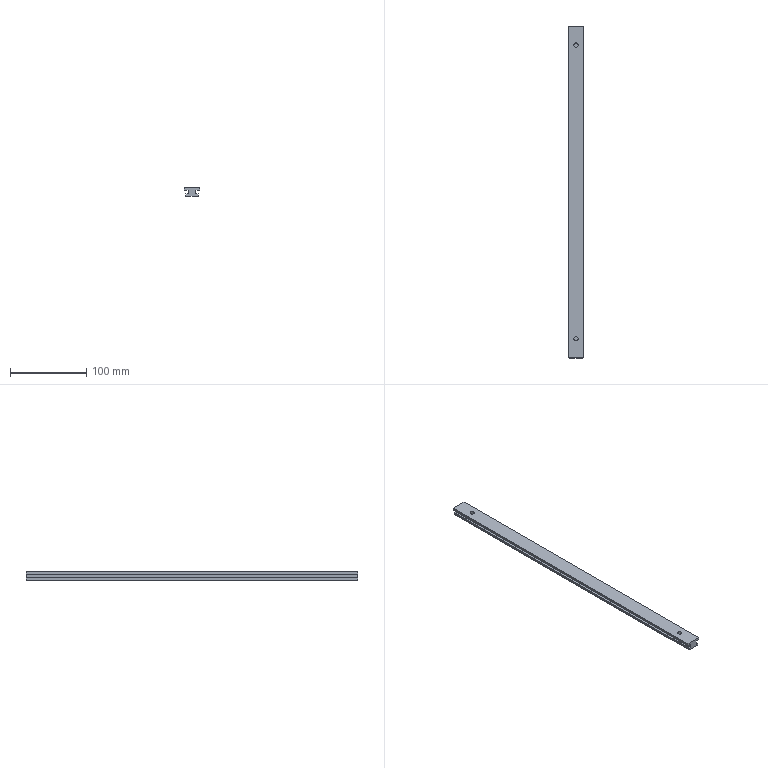Part | SolidWorks | features Extrusion 1, ICE 1 | 1 solid | 20 faces | box 20 x 435 x 11 mm | volume 68492 mm3 | plane 16 | cylinder 4 | commonest cylinder face diameters 5.5 x4
STEP:
#1=CARTESIAN_POINT('',(7.25,410.,-5.));
#2=VERTEX_POINT('',#1);
#3=CARTESIAN_POINT('',(12.75,410.,-5.));
#4=VERTEX_POINT('',#3);
#5=CARTESIAN_POINT('',(10.,410.,-5.));
#6=DIRECTION('',(0.,0.,1.));
#7=DIRECTION('',(1.,0.,0.));
#8=AXIS2_PLACEMENT_3D('',#5,#6,#7);
#9=CIRCLE('',#8,2.75);
#10=EDGE_CURVE('',#2,#4,#9,.T.);
#11=ORIENTED_EDGE('',*,*,#10,.F.);
#12=CARTESIAN_POINT('',(7.25,410.,0.));
#13=VERTEX_POINT('',#12);
#14=CARTESIAN_POINT('',(7.25,410.,-5.));
#15=DIRECTION('',(0.,0.,1.));
#16=VECTOR('',#15,1000.);
#17=LINE('',#14,#16);
#18=EDGE_CURVE('',#2,#13,#17,.T.);
#19=ORIENTED_EDGE('',*,*,#18,.T.);
#20=CARTESIAN_POINT('',(12.75,410.,0.));
#21=VERTEX_POINT('',#20);
#22=CARTESIAN_POINT('',(10.,410.,0.));
#23=DIRECTION('',(0.,0.,1.));
#24=DIRECTION('',(1.,0.,0.));
#25=AXIS2_PLACEMENT_3D('',#22,#23,#24);
#26=CIRCLE('',#25,2.75);
#27=EDGE_CURVE('',#13,#21,#26,.T.);
#28=ORIENTED_EDGE('',*,*,#27,.T.);
#29=CARTESIAN_POINT('',(12.75,410.,-5.));
#30=DIRECTION('',(0.,0.,1.));
#31=VECTOR('',#30,1000.);
#32=LINE('',#29,#31);
#33=EDGE_CURVE('',#4,#21,#32,.T.);
#34=ORIENTED_EDGE('',*,*,#33,.F.);
#35=EDGE_LOOP('',(#11,#19,#28,#34));
#36=FACE_OUTER_BOUND('',#35,.T.);
#37=CARTESIAN_POINT('',(10.,410.,-5.));
#38=DIRECTION('',(0.,0.,1.));
#39=DIRECTION('',(1.,0.,0.));
#40=AXIS2_PLACEMENT_3D('',#37,#38,#39);
#41=CYLINDRICAL_SURFACE('',#40,2.75);
#42=ADVANCED_FACE('',(#36),#41,.F.);
#43=CARTESIAN_POINT('',(7.25,25.,-5.));
#44=VERTEX_POINT('',#43);
#45=CARTESIAN_POINT('',(12.75,25.,-5.));
#46=VERTEX_POINT('',#45);
#47=CARTESIAN_POINT('',(10.,25.,-5.));
#48=DIRECTION('',(0.,0.,1.));
#49=DIRECTION('',(1.,0.,0.));
#50=AXIS2_PLACEMENT_3D('',#47,#48,#49);
#51=CIRCLE('',#50,2.75);
#52=EDGE_CURVE('',#44,#46,#51,.T.);
#53=ORIENTED_EDGE('',*,*,#52,.F.);
#54=CARTESIAN_POINT('',(7.25,25.,0.));
#55=VERTEX_POINT('',#54);
#56=CARTESIAN_POINT('',(7.25,25.,-5.));
#57=DIRECTION('',(0.,0.,1.));
#58=VECTOR('',#57,1000.);
#59=LINE('',#56,#58);
#60=EDGE_CURVE('',#44,#55,#59,.T.);
#61=ORIENTED_EDGE('',*,*,#60,.T.);
#62=CARTESIAN_POINT('',(12.75,25.,0.));
#63=VERTEX_POINT('',#62);
#64=CARTESIAN_POINT('',(10.,25.,0.));
#65=DIRECTION('',(0.,0.,1.));
#66=DIRECTION('',(1.,0.,0.));
#67=AXIS2_PLACEMENT_3D('',#64,#65,#66);
#68=CIRCLE('',#67,2.75);
#69=EDGE_CURVE('',#55,#63,#68,.T.);
#70=ORIENTED_EDGE('',*,*,#69,.T.);
#71=CARTESIAN_POINT('',(12.75,25.,-5.));
#72=DIRECTION('',(0.,0.,1.));
#73=VECTOR('',#72,1000.);
#74=LINE('',#71,#73);
#75=EDGE_CURVE('',#46,#63,#74,.T.);
#76=ORIENTED_EDGE('',*,*,#75,.F.);
#77=EDGE_LOOP('',(#53,#61,#70,#76));
#78=FACE_OUTER_BOUND('',#77,.T.);
#79=CARTESIAN_POINT('',(10.,25.,-5.));
#80=DIRECTION('',(0.,0.,1.));
#81=DIRECTION('',(1.,0.,0.));
#82=AXIS2_PLACEMENT_3D('',#79,#80,#81);
#83=CYLINDRICAL_SURFACE('',#82,2.75);
#84=ADVANCED_FACE('',(#78),#83,.F.);
#85=CARTESIAN_POINT('',(0.,0.,-3.));
#86=VERTEX_POINT('',#85);
#87=CARTESIAN_POINT('',(0.,0.,0.));
#88=VERTEX_POINT('',#87);
#89=CARTESIAN_POINT('',(0.,0.,-3.));
#90=DIRECTION('',(0.,0.,1.));
#91=VECTOR('',#90,1000.);
#92=LINE('',#89,#91);
#93=EDGE_CURVE('',#86,#88,#92,.T.);
#94=ORIENTED_EDGE('',*,*,#93,.T.);
#95=CARTESIAN_POINT('',(0.,435.,0.));
#96=VERTEX_POINT('',#95);
#97=CARTESIAN_POINT('',(0.,435.,0.));
#98=DIRECTION('',(0.,-1.,0.));
#99=VECTOR('',#98,1000.);
#100=LINE('',#97,#99);
#101=EDGE_CURVE('',#96,#88,#100,.T.);
#102=ORIENTED_EDGE('',*,*,#101,.F.);
#103=CARTESIAN_POINT('',(0.,435.,-3.));
#104=VERTEX_POINT('',#103);
#105=CARTESIAN_POINT('',(0.,435.,-3.));
#106=DIRECTION('',(0.,0.,1.));
#107=VECTOR('',#106,1000.);
#108=LINE('',#105,#107);
#109=EDGE_CURVE('',#104,#96,#108,.T.);
#110=ORIENTED_EDGE('',*,*,#109,.F.);
#111=CARTESIAN_POINT('',(0.,435.,-3.));
#112=DIRECTION('',(0.,-1.,0.));
#113=VECTOR('',#112,1000.);
#114=LINE('',#111,#113);
#115=EDGE_CURVE('',#104,#86,#114,.T.);
#116=ORIENTED_EDGE('',*,*,#115,.T.);
#117=EDGE_LOOP('',(#94,#102,#110,#116));
#118=FACE_OUTER_BOUND('',#117,.T.);
#119=CARTESIAN_POINT('',(0.,435.,-3.));
#120=DIRECTION('',(1.,0.,0.));
#121=DIRECTION('',(0.,0.,-1.));
#122=AXIS2_PLACEMENT_3D('',#119,#120,#121);
#123=PLANE('',#122);
#124=ADVANCED_FACE('',(#118),#123,.F.);
#125=CARTESIAN_POINT('',(10.,410.,0.));
#126=DIRECTION('',(0.,0.,1.));
#127=DIRECTION('',(1.,0.,0.));
#128=AXIS2_PLACEMENT_3D('',#125,#126,#127);
#129=CIRCLE('',#128,2.75);
#130=EDGE_CURVE('',#21,#13,#129,.T.);
#131=ORIENTED_EDGE('',*,*,#130,.F.);
#132=ORIENTED_EDGE('',*,*,#27,.F.);
#133=EDGE_LOOP('',(#131,#132));
#134=FACE_BOUND('',#133,.T.);
#135=CARTESIAN_POINT('',(10.,25.,0.));
#136=DIRECTION('',(0.,0.,1.));
#137=DIRECTION('',(1.,0.,0.));
#138=AXIS2_PLACEMENT_3D('',#135,#136,#137);
#139=CIRCLE('',#138,2.75);
#140=EDGE_CURVE('',#63,#55,#139,.T.);
#141=ORIENTED_EDGE('',*,*,#140,.F.);
#142=ORIENTED_EDGE('',*,*,#69,.F.);
#143=EDGE_LOOP('',(#141,#142));
#144=FACE_BOUND('',#143,.T.);
#145=CARTESIAN_POINT('',(20.,0.,0.));
#146=VERTEX_POINT('',#145);
#147=CARTESIAN_POINT('',(0.,0.,0.));
#148=DIRECTION('',(1.,0.,0.));
#149=VECTOR('',#148,1000.);
#150=LINE('',#147,#149);
#151=EDGE_CURVE('',#88,#146,#150,.T.);
#152=ORIENTED_EDGE('',*,*,#151,.T.);
#153=CARTESIAN_POINT('',(20.,435.,0.));
#154=VERTEX_POINT('',#153);
#155=CARTESIAN_POINT('',(20.,435.,0.));
#156=DIRECTION('',(0.,-1.,0.));
#157=VECTOR('',#156,1000.);
#158=LINE('',#155,#157);
#159=EDGE_CURVE('',#154,#146,#158,.T.);
#160=ORIENTED_EDGE('',*,*,#159,.F.);
#161=CARTESIAN_POINT('',(0.,435.,0.));
#162=DIRECTION('',(1.,0.,0.));
#163=VECTOR('',#162,1000.);
#164=LINE('',#161,#163);
#165=EDGE_CURVE('',#96,#154,#164,.T.);
#166=ORIENTED_EDGE('',*,*,#165,.F.);
#167=ORIENTED_EDGE('',*,*,#101,.T.);
#168=EDGE_LOOP('',(#152,#160,#166,#167));
#169=FACE_OUTER_BOUND('',#168,.T.);
#170=CARTESIAN_POINT('',(0.,435.,0.));
#171=DIRECTION('',(0.,0.,-1.));
#172=DIRECTION('',(-1.,0.,0.));
#173=AXIS2_PLACEMENT_3D('',#170,#171,#172);
#174=PLANE('',#173);
#175=ADVANCED_FACE('',(#134,#144,#169),#174,.F.);
#176=CARTESIAN_POINT('',(20.,0.,-3.));
#177=VERTEX_POINT('',#176);
#178=CARTESIAN_POINT('',(20.,0.,0.));
#179=DIRECTION('',(0.,0.,-1.));
#180=VECTOR('',#179,1000.);
#181=LINE('',#178,#180);
#182=EDGE_CURVE('',#146,#177,#181,.T.);
#183=ORIENTED_EDGE('',*,*,#182,.T.);
#184=CARTESIAN_POINT('',(20.,435.,-3.));
#185=VERTEX_POINT('',#184);
#186=CARTESIAN_POINT('',(20.,435.,-3.));
#187=DIRECTION('',(0.,-1.,0.));
#188=VECTOR('',#187,1000.);
#189=LINE('',#186,#188);
#190=EDGE_CURVE('',#185,#177,#189,.T.);
#191=ORIENTED_EDGE('',*,*,#190,.F.);
#192=CARTESIAN_POINT('',(20.,435.,0.));
#193=DIRECTION('',(0.,0.,-1.));
#194=VECTOR('',#193,1000.);
#195=LINE('',#192,#194);
#196=EDGE_CURVE('',#154,#185,#195,.T.);
#197=ORIENTED_EDGE('',*,*,#196,.F.);
#198=ORIENTED_EDGE('',*,*,#159,.T.);
#199=EDGE_LOOP('',(#183,#191,#197,#198));
#200=FACE_OUTER_BOUND('',#199,.T.);
#201=CARTESIAN_POINT('',(20.,435.,0.));
#202=DIRECTION('',(-1.,0.,0.));
#203=DIRECTION('',(0.,0.,1.));
#204=AXIS2_PLACEMENT_3D('',#201,#202,#203);
#205=PLANE('',#204);
#206=ADVANCED_FACE('',(#200),#205,.F.);
#207=CARTESIAN_POINT('',(15.,0.,-3.));
#208=VERTEX_POINT('',#207);
#209=CARTESIAN_POINT('',(20.,0.,-3.));
#210=DIRECTION('',(-1.,0.,0.));
#211=VECTOR('',#210,1000.);
#212=LINE('',#209,#211);
#213=EDGE_CURVE('',#177,#208,#212,.T.);
#214=ORIENTED_EDGE('',*,*,#213,.T.);
#215=CARTESIAN_POINT('',(15.,435.,-3.));
#216=VERTEX_POINT('',#215);
#217=CARTESIAN_POINT('',(15.,435.,-3.));
#218=DIRECTION('',(0.,-1.,0.));
#219=VECTOR('',#218,1000.);
#220=LINE('',#217,#219);
#221=EDGE_CURVE('',#216,#208,#220,.T.);
#222=ORIENTED_EDGE('',*,*,#221,.F.);
#223=CARTESIAN_POINT('',(20.,435.,-3.));
#224=DIRECTION('',(-1.,0.,0.));
#225=VECTOR('',#224,1000.);
#226=LINE('',#223,#225);
#227=EDGE_CURVE('',#185,#216,#226,.T.);
#228=ORIENTED_EDGE('',*,*,#227,.F.);
#229=ORIENTED_EDGE('',*,*,#190,.T.);
#230=EDGE_LOOP('',(#214,#222,#228,#229));
#231=FACE_OUTER_BOUND('',#230,.T.);
#232=CARTESIAN_POINT('',(20.,435.,-3.));
#233=DIRECTION('',(0.,0.,1.));
#234=DIRECTION('',(1.,0.,0.));
#235=AXIS2_PLACEMENT_3D('',#232,#233,#234);
#236=PLANE('',#235);
#237=ADVANCED_FACE('',(#231),#236,.F.);
#238=CARTESIAN_POINT('',(15.,0.,-8.));
#239=VERTEX_POINT('',#238);
#240=CARTESIAN_POINT('',(15.,0.,-3.));
#241=DIRECTION('',(0.,0.,-1.));
#242=VECTOR('',#241,1000.);
#243=LINE('',#240,#242);
#244=EDGE_CURVE('',#208,#239,#243,.T.);
#245=ORIENTED_EDGE('',*,*,#244,.T.);
#246=CARTESIAN_POINT('',(15.,435.,-8.));
#247=VERTEX_POINT('',#246);
#248=CARTESIAN_POINT('',(15.,435.,-8.));
#249=DIRECTION('',(0.,-1.,0.));
#250=VECTOR('',#249,1000.);
#251=LINE('',#248,#250);
#252=EDGE_CURVE('',#247,#239,#251,.T.);
#253=ORIENTED_EDGE('',*,*,#252,.F.);
#254=CARTESIAN_POINT('',(15.,435.,-3.));
#255=DIRECTION('',(0.,0.,-1.));
#256=VECTOR('',#255,1000.);
#257=LINE('',#254,#256);
#258=EDGE_CURVE('',#216,#247,#257,.T.);
#259=ORIENTED_EDGE('',*,*,#258,.F.);
#260=ORIENTED_EDGE('',*,*,#221,.T.);
#261=EDGE_LOOP('',(#245,#253,#259,#260));
#262=FACE_OUTER_BOUND('',#261,.T.);
#263=CARTESIAN_POINT('',(15.,435.,-3.));
#264=DIRECTION('',(-1.,0.,0.));
#265=DIRECTION('',(0.,0.,1.));
#266=AXIS2_PLACEMENT_3D('',#263,#264,#265);
#267=PLANE('',#266);
#268=ADVANCED_FACE('',(#262),#267,.F.);
#269=CARTESIAN_POINT('',(18.,0.,-8.));
#270=VERTEX_POINT('',#269);
#271=CARTESIAN_POINT('',(15.,0.,-8.));
#272=DIRECTION('',(1.,0.,0.));
#273=VECTOR('',#272,1000.);
#274=LINE('',#271,#273);
#275=EDGE_CURVE('',#239,#270,#274,.T.);
#276=ORIENTED_EDGE('',*,*,#275,.T.);
#277=CARTESIAN_POINT('',(18.,435.,-8.));
#278=VERTEX_POINT('',#277);
#279=CARTESIAN_POINT('',(18.,435.,-8.));
#280=DIRECTION('',(0.,-1.,0.));
#281=VECTOR('',#280,1000.);
#282=LINE('',#279,#281);
#283=EDGE_CURVE('',#278,#270,#282,.T.);
#284=ORIENTED_EDGE('',*,*,#283,.F.);
#285=CARTESIAN_POINT('',(15.,435.,-8.));
#286=DIRECTION('',(1.,0.,0.));
#287=VECTOR('',#286,1000.);
#288=LINE('',#285,#287);
#289=EDGE_CURVE('',#247,#278,#288,.T.);
#290=ORIENTED_EDGE('',*,*,#289,.F.);
#291=ORIENTED_EDGE('',*,*,#252,.T.);
#292=EDGE_LOOP('',(#276,#284,#290,#291));
#293=FACE_OUTER_BOUND('',#292,.T.);
#294=CARTESIAN_POINT('',(15.,435.,-8.));
#295=DIRECTION('',(0.,0.,-1.));
#296=DIRECTION('',(-1.,0.,0.));
#297=AXIS2_PLACEMENT_3D('',#294,#295,#296);
#298=PLANE('',#297);
#299=ADVANCED_FACE('',(#293),#298,.F.);
#300=CARTESIAN_POINT('',(18.,0.,-11.));
#301=VERTEX_POINT('',#300);
#302=CARTESIAN_POINT('',(18.,0.,-8.));
#303=DIRECTION('',(0.,0.,-1.));
#304=VECTOR('',#303,1000.);
#305=LINE('',#302,#304);
#306=EDGE_CURVE('',#270,#301,#305,.T.);
#307=ORIENTED_EDGE('',*,*,#306,.T.);
#308=CARTESIAN_POINT('',(18.,435.,-11.));
#309=VERTEX_POINT('',#308);
#310=CARTESIAN_POINT('',(18.,435.,-11.));
#311=DIRECTION('',(0.,-1.,0.));
#312=VECTOR('',#311,1000.);
#313=LINE('',#310,#312);
#314=EDGE_CURVE('',#309,#301,#313,.T.);
#315=ORIENTED_EDGE('',*,*,#314,.F.);
#316=CARTESIAN_POINT('',(18.,435.,-8.));
#317=DIRECTION('',(0.,0.,-1.));
#318=VECTOR('',#317,1000.);
#319=LINE('',#316,#318);
#320=EDGE_CURVE('',#278,#309,#319,.T.);
#321=ORIENTED_EDGE('',*,*,#320,.F.);
#322=ORIENTED_EDGE('',*,*,#283,.T.);
#323=EDGE_LOOP('',(#307,#315,#321,#322));
#324=FACE_OUTER_BOUND('',#323,.T.);
#325=CARTESIAN_POINT('',(18.,435.,-8.));
#326=DIRECTION('',(-1.,0.,0.));
#327=DIRECTION('',(0.,0.,1.));
#328=AXIS2_PLACEMENT_3D('',#325,#326,#327);
#329=PLANE('',#328);
#330=ADVANCED_FACE('',(#324),#329,.F.);
#331=CARTESIAN_POINT('',(2.,0.,-11.));
#332=VERTEX_POINT('',#331);
#333=CARTESIAN_POINT('',(18.,0.,-11.));
#334=DIRECTION('',(-1.,0.,0.));
#335=VECTOR('',#334,1000.);
#336=LINE('',#333,#335);
#337=EDGE_CURVE('',#301,#332,#336,.T.);
#338=ORIENTED_EDGE('',*,*,#337,.T.);
#339=CARTESIAN_POINT('',(2.,435.,-11.));
#340=VERTEX_POINT('',#339);
#341=CARTESIAN_POINT('',(2.,435.,-11.));
#342=DIRECTION('',(0.,-1.,0.));
#343=VECTOR('',#342,1000.);
#344=LINE('',#341,#343);
#345=EDGE_CURVE('',#340,#332,#344,.T.);
#346=ORIENTED_EDGE('',*,*,#345,.F.);
#347=CARTESIAN_POINT('',(18.,435.,-11.));
#348=DIRECTION('',(-1.,0.,0.));
#349=VECTOR('',#348,1000.);
#350=LINE('',#347,#349);
#351=EDGE_CURVE('',#309,#340,#350,.T.);
#352=ORIENTED_EDGE('',*,*,#351,.F.);
#353=ORIENTED_EDGE('',*,*,#314,.T.);
#354=EDGE_LOOP('',(#338,#346,#352,#353));
#355=FACE_OUTER_BOUND('',#354,.T.);
#356=CARTESIAN_POINT('',(18.,435.,-11.));
#357=DIRECTION('',(0.,0.,1.));
#358=DIRECTION('',(1.,0.,0.));
#359=AXIS2_PLACEMENT_3D('',#356,#357,#358);
#360=PLANE('',#359);
#361=ADVANCED_FACE('',(#355),#360,.F.);
#362=CARTESIAN_POINT('',(2.,0.,-8.));
#363=VERTEX_POINT('',#362);
#364=CARTESIAN_POINT('',(2.,0.,-11.));
#365=DIRECTION('',(0.,0.,1.));
#366=VECTOR('',#365,1000.);
#367=LINE('',#364,#366);
#368=EDGE_CURVE('',#332,#363,#367,.T.);
#369=ORIENTED_EDGE('',*,*,#368,.T.);
#370=CARTESIAN_POINT('',(2.,435.,-8.));
#371=VERTEX_POINT('',#370);
#372=CARTESIAN_POINT('',(2.,435.,-8.));
#373=DIRECTION('',(0.,-1.,0.));
#374=VECTOR('',#373,1000.);
#375=LINE('',#372,#374);
#376=EDGE_CURVE('',#371,#363,#375,.T.);
#377=ORIENTED_EDGE('',*,*,#376,.F.);
#378=CARTESIAN_POINT('',(2.,435.,-11.));
#379=DIRECTION('',(0.,0.,1.));
#380=VECTOR('',#379,1000.);
#381=LINE('',#378,#380);
#382=EDGE_CURVE('',#340,#371,#381,.T.);
#383=ORIENTED_EDGE('',*,*,#382,.F.);
#384=ORIENTED_EDGE('',*,*,#345,.T.);
#385=EDGE_LOOP('',(#369,#377,#383,#384));
#386=FACE_OUTER_BOUND('',#385,.T.);
#387=CARTESIAN_POINT('',(2.,435.,-11.));
#388=DIRECTION('',(1.,0.,0.));
#389=DIRECTION('',(0.,0.,-1.));
#390=AXIS2_PLACEMENT_3D('',#387,#388,#389);
#391=PLANE('',#390);
#392=ADVANCED_FACE('',(#386),#391,.F.);
#393=CARTESIAN_POINT('',(5.,0.,-8.));
#394=VERTEX_POINT('',#393);
#395=CARTESIAN_POINT('',(2.,0.,-8.));
#396=DIRECTION('',(1.,0.,0.));
#397=VECTOR('',#396,1000.);
#398=LINE('',#395,#397);
#399=EDGE_CURVE('',#363,#394,#398,.T.);
#400=ORIENTED_EDGE('',*,*,#399,.T.);
#401=CARTESIAN_POINT('',(5.,435.,-8.));
#402=VERTEX_POINT('',#401);
#403=CARTESIAN_POINT('',(5.,435.,-8.));
#404=DIRECTION('',(0.,-1.,0.));
#405=VECTOR('',#404,1000.);
#406=LINE('',#403,#405);
#407=EDGE_CURVE('',#402,#394,#406,.T.);
#408=ORIENTED_EDGE('',*,*,#407,.F.);
#409=CARTESIAN_POINT('',(2.,435.,-8.));
#410=DIRECTION('',(1.,0.,0.));
#411=VECTOR('',#410,1000.);
#412=LINE('',#409,#411);
#413=EDGE_CURVE('',#371,#402,#412,.T.);
#414=ORIENTED_EDGE('',*,*,#413,.F.);
#415=ORIENTED_EDGE('',*,*,#376,.T.);
#416=EDGE_LOOP('',(#400,#408,#414,#415));
#417=FACE_OUTER_BOUND('',#416,.T.);
#418=CARTESIAN_POINT('',(2.,435.,-8.));
#419=DIRECTION('',(0.,0.,-1.));
#420=DIRECTION('',(-1.,0.,0.));
#421=AXIS2_PLACEMENT_3D('',#418,#419,#420);
#422=PLANE('',#421);
#423=ADVANCED_FACE('',(#417),#422,.F.);
#424=CARTESIAN_POINT('',(5.,0.,-3.));
#425=VERTEX_POINT('',#424);
#426=CARTESIAN_POINT('',(5.,0.,-8.));
#427=DIRECTION('',(0.,0.,1.));
#428=VECTOR('',#427,1000.);
#429=LINE('',#426,#428);
#430=EDGE_CURVE('',#394,#425,#429,.T.);
#431=ORIENTED_EDGE('',*,*,#430,.T.);
#432=CARTESIAN_POINT('',(5.,435.,-3.));
#433=VERTEX_POINT('',#432);
#434=CARTESIAN_POINT('',(5.,435.,-3.));
#435=DIRECTION('',(0.,-1.,0.));
#436=VECTOR('',#435,1000.);
#437=LINE('',#434,#436);
#438=EDGE_CURVE('',#433,#425,#437,.T.);
#439=ORIENTED_EDGE('',*,*,#438,.F.);
#440=CARTESIAN_POINT('',(5.,435.,-8.));
#441=DIRECTION('',(0.,0.,1.));
#442=VECTOR('',#441,1000.);
#443=LINE('',#440,#442);
#444=EDGE_CURVE('',#402,#433,#443,.T.);
#445=ORIENTED_EDGE('',*,*,#444,.F.);
#446=ORIENTED_EDGE('',*,*,#407,.T.);
#447=EDGE_LOOP('',(#431,#439,#445,#446));
#448=FACE_OUTER_BOUND('',#447,.T.);
#449=CARTESIAN_POINT('',(5.,435.,-8.));
#450=DIRECTION('',(1.,0.,0.));
#451=DIRECTION('',(0.,0.,-1.));
#452=AXIS2_PLACEMENT_3D('',#449,#450,#451);
#453=PLANE('',#452);
#454=ADVANCED_FACE('',(#448),#453,.F.);
#455=CARTESIAN_POINT('',(5.,0.,-3.));
#456=DIRECTION('',(-1.,0.,0.));
#457=VECTOR('',#456,1000.);
#458=LINE('',#455,#457);
#459=EDGE_CURVE('',#425,#86,#458,.T.);
#460=ORIENTED_EDGE('',*,*,#459,.T.);
#461=ORIENTED_EDGE('',*,*,#115,.F.);
#462=CARTESIAN_POINT('',(5.,435.,-3.));
#463=DIRECTION('',(-1.,0.,0.));
#464=VECTOR('',#463,1000.);
#465=LINE('',#462,#464);
#466=EDGE_CURVE('',#433,#104,#465,.T.);
#467=ORIENTED_EDGE('',*,*,#466,.F.);
#468=ORIENTED_EDGE('',*,*,#438,.T.);
#469=EDGE_LOOP('',(#460,#461,#467,#468));
#470=FACE_OUTER_BOUND('',#469,.T.);
#471=CARTESIAN_POINT('',(5.,435.,-3.));
#472=DIRECTION('',(0.,0.,1.));
#473=DIRECTION('',(1.,0.,0.));
#474=AXIS2_PLACEMENT_3D('',#471,#472,#473);
#475=PLANE('',#474);
#476=ADVANCED_FACE('',(#470),#475,.F.);
#477=ORIENTED_EDGE('',*,*,#109,.T.);
#478=ORIENTED_EDGE('',*,*,#165,.T.);
#479=ORIENTED_EDGE('',*,*,#196,.T.);
#480=ORIENTED_EDGE('',*,*,#227,.T.);
#481=ORIENTED_EDGE('',*,*,#258,.T.);
#482=ORIENTED_EDGE('',*,*,#289,.T.);
#483=ORIENTED_EDGE('',*,*,#320,.T.);
#484=ORIENTED_EDGE('',*,*,#351,.T.);
#485=ORIENTED_EDGE('',*,*,#382,.T.);
#486=ORIENTED_EDGE('',*,*,#413,.T.);
#487=ORIENTED_EDGE('',*,*,#444,.T.);
#488=ORIENTED_EDGE('',*,*,#466,.T.);
#489=EDGE_LOOP('',(#477,#478,#479,#480,#481,#482,#483,#484,#485,#486,#487,#488));
#490=FACE_OUTER_BOUND('',#489,.T.);
#491=CARTESIAN_POINT('',(0.,435.,0.));
#492=DIRECTION('',(0.,1.,0.));
#493=DIRECTION('',(0.,0.,1.));
#494=AXIS2_PLACEMENT_3D('',#491,#492,#493);
#495=PLANE('',#494);
#496=ADVANCED_FACE('',(#490),#495,.T.);
#497=ORIENTED_EDGE('',*,*,#93,.F.);
#498=ORIENTED_EDGE('',*,*,#459,.F.);
#499=ORIENTED_EDGE('',*,*,#430,.F.);
#500=ORIENTED_EDGE('',*,*,#399,.F.);
#501=ORIENTED_EDGE('',*,*,#368,.F.);
#502=ORIENTED_EDGE('',*,*,#337,.F.);
#503=ORIENTED_EDGE('',*,*,#306,.F.);
#504=ORIENTED_EDGE('',*,*,#275,.F.);
#505=ORIENTED_EDGE('',*,*,#244,.F.);
#506=ORIENTED_EDGE('',*,*,#213,.F.);
#507=ORIENTED_EDGE('',*,*,#182,.F.);
#508=ORIENTED_EDGE('',*,*,#151,.F.);
#509=EDGE_LOOP('',(#497,#498,#499,#500,#501,#502,#503,#504,#505,#506,#507,#508));
#510=FACE_OUTER_BOUND('',#509,.T.);
#511=CARTESIAN_POINT('',(0.,0.,0.));
#512=DIRECTION('',(0.,1.,0.));
#513=DIRECTION('',(0.,0.,1.));
#514=AXIS2_PLACEMENT_3D('',#511,#512,#513);
#515=PLANE('',#514);
#516=ADVANCED_FACE('',(#510),#515,.F.);
#517=ORIENTED_EDGE('',*,*,#60,.F.);
#518=CARTESIAN_POINT('',(10.,25.,-5.));
#519=DIRECTION('',(0.,0.,1.));
#520=DIRECTION('',(1.,0.,0.));
#521=AXIS2_PLACEMENT_3D('',#518,#519,#520);
#522=CIRCLE('',#521,2.75);
#523=EDGE_CURVE('',#46,#44,#522,.T.);
#524=ORIENTED_EDGE('',*,*,#523,.F.);
#525=ORIENTED_EDGE('',*,*,#75,.T.);
#526=ORIENTED_EDGE('',*,*,#140,.T.);
#527=EDGE_LOOP('',(#517,#524,#525,#526));
#528=FACE_OUTER_BOUND('',#527,.T.);
#529=CARTESIAN_POINT('',(10.,25.,-5.));
#530=DIRECTION('',(0.,0.,1.));
#531=DIRECTION('',(1.,0.,0.));
#532=AXIS2_PLACEMENT_3D('',#529,#530,#531);
#533=CYLINDRICAL_SURFACE('',#532,2.75);
#534=ADVANCED_FACE('',(#528),#533,.F.);
#535=ORIENTED_EDGE('',*,*,#523,.T.);
#536=ORIENTED_EDGE('',*,*,#52,.T.);
#537=EDGE_LOOP('',(#535,#536));
#538=FACE_OUTER_BOUND('',#537,.T.);
#539=CARTESIAN_POINT('',(10.,25.,-5.));
#540=DIRECTION('',(0.,0.,1.));
#541=DIRECTION('',(1.,0.,0.));
#542=AXIS2_PLACEMENT_3D('',#539,#540,#541);
#543=PLANE('',#542);
#544=ADVANCED_FACE('',(#538),#543,.T.);
#545=ORIENTED_EDGE('',*,*,#18,.F.);
#546=CARTESIAN_POINT('',(10.,410.,-5.));
#547=DIRECTION('',(0.,0.,1.));
#548=DIRECTION('',(1.,0.,0.));
#549=AXIS2_PLACEMENT_3D('',#546,#547,#548);
#550=CIRCLE('',#549,2.75);
#551=EDGE_CURVE('',#4,#2,#550,.T.);
#552=ORIENTED_EDGE('',*,*,#551,.F.);
#553=ORIENTED_EDGE('',*,*,#33,.T.);
#554=ORIENTED_EDGE('',*,*,#130,.T.);
#555=EDGE_LOOP('',(#545,#552,#553,#554));
#556=FACE_OUTER_BOUND('',#555,.T.);
#557=CARTESIAN_POINT('',(10.,410.,-5.));
#558=DIRECTION('',(0.,0.,1.));
#559=DIRECTION('',(1.,0.,0.));
#560=AXIS2_PLACEMENT_3D('',#557,#558,#559);
#561=CYLINDRICAL_SURFACE('',#560,2.75);
#562=ADVANCED_FACE('',(#556),#561,.F.);
#563=ORIENTED_EDGE('',*,*,#551,.T.);
#564=ORIENTED_EDGE('',*,*,#10,.T.);
#565=EDGE_LOOP('',(#563,#564));
#566=FACE_OUTER_BOUND('',#565,.T.);
#567=CARTESIAN_POINT('',(10.,410.,-5.));
#568=DIRECTION('',(0.,0.,1.));
#569=DIRECTION('',(1.,0.,0.));
#570=AXIS2_PLACEMENT_3D('',#567,#568,#569);
#571=PLANE('',#570);
#572=ADVANCED_FACE('',(#566),#571,.T.);
#573=CLOSED_SHELL('',(#42,#84,#124,#175,#206,#237,#268,#299,#330,#361,#392,#423,#454,#476,#496,#516,#534,#544,#562,#572));
#574=MANIFOLD_SOLID_BREP('',#573);
#575=CARTESIAN_POINT('',(0.,0.,0.));
#576=DIRECTION('',(0.,0.,1.));
#577=DIRECTION('',(1.,0.,0.));
#578=AXIS2_PLACEMENT_3D('',#575,#576,#577);
#579=(LENGTH_UNIT()NAMED_UNIT(*)SI_UNIT(.MILLI.,.METRE.));
#580=UNCERTAINTY_MEASURE_WITH_UNIT(LENGTH_MEASURE(0.00001),#579,'','');
#581=(NAMED_UNIT(*)PLANE_ANGLE_UNIT()SI_UNIT($,.RADIAN.));
#582=(NAMED_UNIT(*)SI_UNIT($,.STERADIAN.)SOLID_ANGLE_UNIT());
#583=(GEOMETRIC_REPRESENTATION_CONTEXT(3)GLOBAL_UNCERTAINTY_ASSIGNED_CONTEXT((#580))GLOBAL_UNIT_ASSIGNED_CONTEXT((#579,#581,#582))REPRESENTATION_CONTEXT('',''));
#584=ADVANCED_BREP_SHAPE_REPRESENTATION('',(#574,#578),#583);